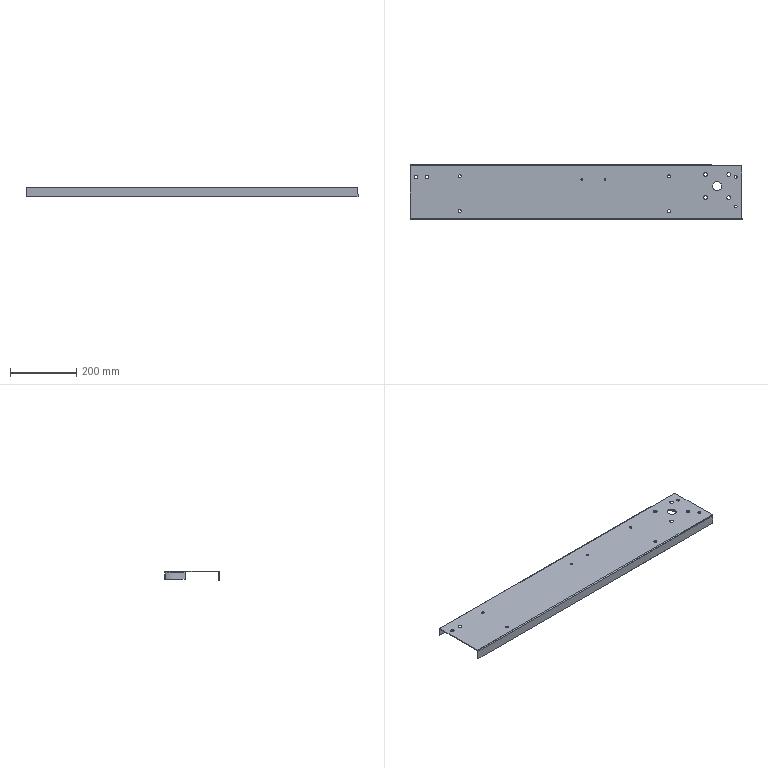Part | SolidWorks | features BaseBody 1 | 1 solid | 53 faces | box 1000 x 165 x 30 mm | volume 425312 mm3 | cylinder 36 | plane 16 | spline 1 | commonest cylinder face diameters 8.5 x12 11.5 x8 5.5 x4 11 x4 1.473 x2 5.473 x2